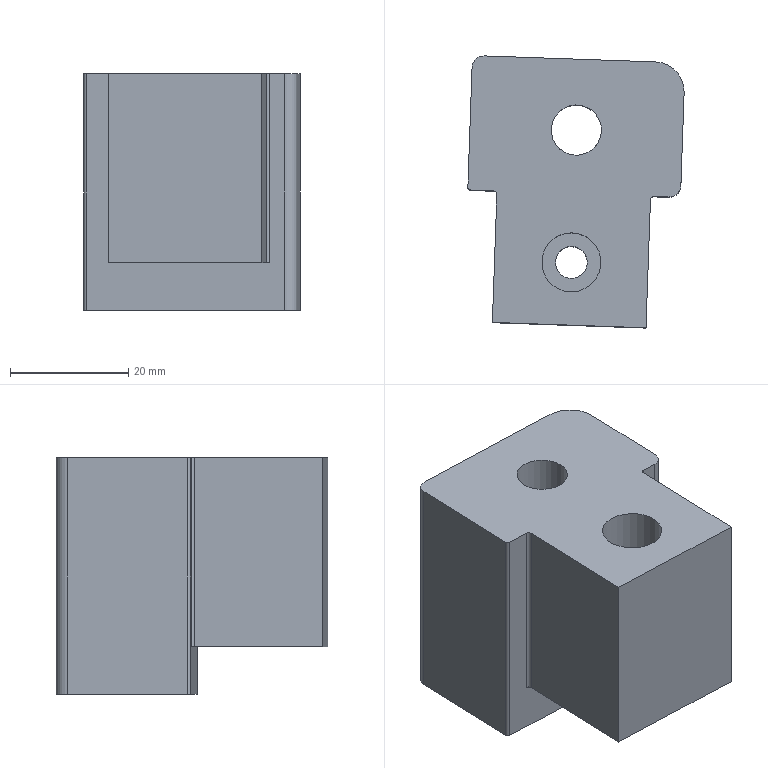Part | NX | features PS-25 2 | 1 solid | 22 faces | box 36.584 x 45.984 x 40 mm | volume 45378 mm3 | plane 12 | cylinder 10 | commonest cylinder face diameters 1 x3 4 x2 10 x2 5.4 x1 8.506 x1 14.5 x1
STEP:
#1=CARTESIAN_POINT('',(3172.903,-916.865,868.716));
#2=VERTEX_POINT('',#1);
#3=CARTESIAN_POINT('',(3198.887,-917.772,868.716));
#4=VERTEX_POINT('',#3);
#5=CARTESIAN_POINT('',(3185.895,-917.319,868.716));
#6=DIRECTION('',(0.9994,-0.0349,0.));
#7=VECTOR('',#6,1000.);
#8=LINE('',#5,#7);
#9=EDGE_CURVE('',#2,#4,#8,.T.);
#10=ORIENTED_EDGE('',*,*,#9,.F.);
#11=CARTESIAN_POINT('',(3173.662,-895.141,868.716));
#12=VERTEX_POINT('',#11);
#13=CARTESIAN_POINT('',(3172.937,-915.898,868.716));
#14=DIRECTION('',(-0.0349,-0.9994,0.));
#15=VECTOR('',#14,1000.);
#16=LINE('',#13,#15);
#17=EDGE_CURVE('',#2,#12,#16,.F.);
#18=ORIENTED_EDGE('',*,*,#17,.T.);
#19=CARTESIAN_POINT('',(3173.179,-894.624,868.716));
#20=VERTEX_POINT('',#19);
#21=CARTESIAN_POINT('',(3173.162,-895.124,868.716));
#22=DIRECTION('',(0.,0.,-1.));
#23=DIRECTION('',(-1.,0.,0.));
#24=AXIS2_PLACEMENT_3D('',#21,#22,#23);
#25=CIRCLE('',#24,0.5);
#26=EDGE_CURVE('',#12,#20,#25,.F.);
#27=ORIENTED_EDGE('',*,*,#26,.T.);
#28=CARTESIAN_POINT('',(3200.163,-895.566,868.716));
#29=VERTEX_POINT('',#28);
#30=CARTESIAN_POINT('',(3186.671,-895.095,868.716));
#31=DIRECTION('',(0.9994,-0.0349,0.));
#32=VECTOR('',#31,1000.);
#33=LINE('',#30,#32);
#34=EDGE_CURVE('',#20,#29,#33,.T.);
#35=ORIENTED_EDGE('',*,*,#34,.T.);
#36=CARTESIAN_POINT('',(3199.646,-896.049,868.716));
#37=VERTEX_POINT('',#36);
#38=CARTESIAN_POINT('',(3200.145,-896.066,868.716));
#39=DIRECTION('',(0.,0.,-1.));
#40=DIRECTION('',(-1.,0.,0.));
#41=AXIS2_PLACEMENT_3D('',#38,#39,#40);
#42=CIRCLE('',#41,0.5);
#43=EDGE_CURVE('',#29,#37,#42,.F.);
#44=ORIENTED_EDGE('',*,*,#43,.T.);
#45=CARTESIAN_POINT('',(3198.921,-916.805,868.716));
#46=DIRECTION('',(0.0349,0.9994,0.));
#47=VECTOR('',#46,1000.);
#48=LINE('',#45,#47);
#49=EDGE_CURVE('',#4,#37,#48,.T.);
#50=ORIENTED_EDGE('',*,*,#49,.F.);
#51=EDGE_LOOP('',(#10,#18,#27,#35,#44,#50));
#52=FACE_BOUND('',#51,.T.);
#53=CARTESIAN_POINT('',(3183.566,-906.707,868.716));
#54=VERTEX_POINT('',#53);
#55=CARTESIAN_POINT('',(3186.266,-906.707,868.716));
#56=DIRECTION('',(0.,0.,-1.));
#57=DIRECTION('',(-1.,0.,0.));
#58=AXIS2_PLACEMENT_3D('',#55,#56,#57);
#59=CIRCLE('',#58,2.7);
#60=EDGE_CURVE('',#54,#54,#59,.F.);
#61=ORIENTED_EDGE('',*,*,#60,.T.);
#62=EDGE_LOOP('',(#61));
#63=FACE_BOUND('',#62,.T.);
#64=CARTESIAN_POINT('',(3186.266,-906.707,868.716));
#65=DIRECTION('',(0.,0.,-1.));
#66=DIRECTION('',(-0.0349,-0.9994,0.));
#67=AXIS2_PLACEMENT_3D('',#64,#65,#66);
#68=PLANE('',#67);
#69=ADVANCED_FACE('',(#52,#63),#68,.T.);
#70=CARTESIAN_POINT('',(3186.266,-911.707,900.716));
#71=VERTEX_POINT('',#70);
#72=CARTESIAN_POINT('',(3186.266,-906.707,900.716));
#73=DIRECTION('',(0.,0.,1.));
#74=DIRECTION('',(0.,-1.,0.));
#75=AXIS2_PLACEMENT_3D('',#72,#73,#74);
#76=CIRCLE('',#75,5.);
#77=EDGE_CURVE('',#71,#71,#76,.T.);
#78=ORIENTED_EDGE('',*,*,#77,.F.);
#79=EDGE_LOOP('',(#78));
#80=FACE_BOUND('',#79,.T.);
#81=CARTESIAN_POINT('',(3200.163,-895.566,900.716));
#82=VERTEX_POINT('',#81);
#83=CARTESIAN_POINT('',(3202.722,-895.656,900.716));
#84=VERTEX_POINT('',#83);
#85=CARTESIAN_POINT('',(3027.832,-889.549,900.716));
#86=DIRECTION('',(-0.9994,0.0349,0.));
#87=VECTOR('',#86,1000.);
#88=LINE('',#85,#87);
#89=EDGE_CURVE('',#82,#84,#88,.F.);
#90=ORIENTED_EDGE('',*,*,#89,.T.);
#91=CARTESIAN_POINT('',(3204.79,-893.727,900.716));
#92=VERTEX_POINT('',#91);
#93=CARTESIAN_POINT('',(3202.792,-893.657,900.716));
#94=DIRECTION('',(0.,0.,1.));
#95=DIRECTION('',(0.,-1.,0.));
#96=AXIS2_PLACEMENT_3D('',#93,#94,#95);
#97=CIRCLE('',#96,2.);
#98=EDGE_CURVE('',#84,#92,#97,.T.);
#99=ORIENTED_EDGE('',*,*,#98,.T.);
#100=CARTESIAN_POINT('',(3205.34,-877.973,900.716));
#101=VERTEX_POINT('',#100);
#102=CARTESIAN_POINT('',(3202.812,-950.375,900.716));
#103=DIRECTION('',(-0.0349,-0.9994,0.));
#104=VECTOR('',#103,1000.);
#105=LINE('',#102,#104);
#106=EDGE_CURVE('',#92,#101,#105,.F.);
#107=ORIENTED_EDGE('',*,*,#106,.T.);
#108=CARTESIAN_POINT('',(3200.518,-872.802,900.716));
#109=VERTEX_POINT('',#108);
#110=CARTESIAN_POINT('',(3200.343,-877.799,900.716));
#111=DIRECTION('',(0.,0.,1.));
#112=DIRECTION('',(0.,-1.,0.));
#113=AXIS2_PLACEMENT_3D('',#110,#111,#112);
#114=CIRCLE('',#113,5.);
#115=EDGE_CURVE('',#109,#101,#114,.F.);
#116=ORIENTED_EDGE('',*,*,#115,.F.);
#117=CARTESIAN_POINT('',(3171.536,-871.79,900.716));
#118=VERTEX_POINT('',#117);
#119=CARTESIAN_POINT('',(3158.544,-871.336,900.716));
#120=DIRECTION('',(-0.9994,0.0349,0.));
#121=VECTOR('',#120,1000.);
#122=LINE('',#119,#121);
#123=EDGE_CURVE('',#109,#118,#122,.T.);
#124=ORIENTED_EDGE('',*,*,#123,.T.);
#125=CARTESIAN_POINT('',(3169.467,-873.719,900.716));
#126=VERTEX_POINT('',#125);
#127=CARTESIAN_POINT('',(3171.466,-873.789,900.716));
#128=DIRECTION('',(0.,0.,1.));
#129=DIRECTION('',(0.,-1.,0.));
#130=AXIS2_PLACEMENT_3D('',#127,#128,#129);
#131=CIRCLE('',#130,2.);
#132=EDGE_CURVE('',#126,#118,#131,.F.);
#133=ORIENTED_EDGE('',*,*,#132,.F.);
#134=CARTESIAN_POINT('',(3168.76,-893.97,900.716));
#135=VERTEX_POINT('',#134);
#136=CARTESIAN_POINT('',(3166.834,-949.119,900.716));
#137=DIRECTION('',(-0.0349,-0.9994,0.));
#138=VECTOR('',#137,1000.);
#139=LINE('',#136,#138);
#140=EDGE_CURVE('',#135,#126,#139,.F.);
#141=ORIENTED_EDGE('',*,*,#140,.F.);
#142=CARTESIAN_POINT('',(3169.242,-894.487,900.716));
#143=VERTEX_POINT('',#142);
#144=CARTESIAN_POINT('',(3169.26,-893.987,900.716));
#145=DIRECTION('',(0.,0.,1.));
#146=DIRECTION('',(0.,-1.,0.));
#147=AXIS2_PLACEMENT_3D('',#144,#145,#146);
#148=CIRCLE('',#147,0.5);
#149=EDGE_CURVE('',#135,#143,#148,.T.);
#150=ORIENTED_EDGE('',*,*,#149,.T.);
#151=CARTESIAN_POINT('',(3173.179,-894.624,900.716));
#152=VERTEX_POINT('',#151);
#153=CARTESIAN_POINT('',(3027.832,-889.549,900.716));
#154=DIRECTION('',(-0.9994,0.0349,0.));
#155=VECTOR('',#154,1000.);
#156=LINE('',#153,#155);
#157=EDGE_CURVE('',#143,#152,#156,.F.);
#158=ORIENTED_EDGE('',*,*,#157,.T.);
#159=CARTESIAN_POINT('',(3173.662,-895.141,900.716));
#160=VERTEX_POINT('',#159);
#161=CARTESIAN_POINT('',(3173.162,-895.124,900.716));
#162=DIRECTION('',(0.,0.,1.));
#163=DIRECTION('',(0.,-1.,0.));
#164=AXIS2_PLACEMENT_3D('',#161,#162,#163);
#165=CIRCLE('',#164,0.5);
#166=EDGE_CURVE('',#152,#160,#165,.F.);
#167=ORIENTED_EDGE('',*,*,#166,.T.);
#168=CARTESIAN_POINT('',(3172.903,-916.865,900.716));
#169=VERTEX_POINT('',#168);
#170=CARTESIAN_POINT('',(3172.937,-915.898,900.716));
#171=DIRECTION('',(0.0349,0.9994,0.));
#172=VECTOR('',#171,1000.);
#173=LINE('',#170,#172);
#174=EDGE_CURVE('',#169,#160,#173,.T.);
#175=ORIENTED_EDGE('',*,*,#174,.F.);
#176=CARTESIAN_POINT('',(3198.887,-917.772,900.716));
#177=VERTEX_POINT('',#176);
#178=CARTESIAN_POINT('',(3027.056,-911.773,900.716));
#179=DIRECTION('',(-0.9994,0.0349,0.));
#180=VECTOR('',#179,1000.);
#181=LINE('',#178,#180);
#182=EDGE_CURVE('',#169,#177,#181,.F.);
#183=ORIENTED_EDGE('',*,*,#182,.T.);
#184=CARTESIAN_POINT('',(3199.646,-896.049,900.716));
#185=VERTEX_POINT('',#184);
#186=CARTESIAN_POINT('',(3198.921,-916.805,900.716));
#187=DIRECTION('',(-0.0349,-0.9994,0.));
#188=VECTOR('',#187,1000.);
#189=LINE('',#186,#188);
#190=EDGE_CURVE('',#177,#185,#189,.F.);
#191=ORIENTED_EDGE('',*,*,#190,.T.);
#192=CARTESIAN_POINT('',(3200.145,-896.066,900.716));
#193=DIRECTION('',(0.,0.,1.));
#194=DIRECTION('',(0.,-1.,0.));
#195=AXIS2_PLACEMENT_3D('',#192,#193,#194);
#196=CIRCLE('',#195,0.5);
#197=EDGE_CURVE('',#185,#82,#196,.F.);
#198=ORIENTED_EDGE('',*,*,#197,.T.);
#199=EDGE_LOOP('',(#90,#99,#107,#116,#124,#133,#141,#150,#158,#167,#175,#183,#191,#198));
#200=FACE_BOUND('',#199,.T.);
#201=CARTESIAN_POINT('',(3187.107,-888.594,900.716));
#202=VERTEX_POINT('',#201);
#203=CARTESIAN_POINT('',(3187.107,-884.341,900.716));
#204=DIRECTION('',(0.,0.,1.));
#205=DIRECTION('',(0.,-1.,0.));
#206=AXIS2_PLACEMENT_3D('',#203,#204,#205);
#207=CIRCLE('',#206,4.253);
#208=EDGE_CURVE('',#202,#202,#207,.T.);
#209=ORIENTED_EDGE('',*,*,#208,.F.);
#210=EDGE_LOOP('',(#209));
#211=FACE_BOUND('',#210,.T.);
#212=CARTESIAN_POINT('',(3025.924,-944.199,900.716));
#213=DIRECTION('',(0.,0.,1.));
#214=DIRECTION('',(0.9976,-0.06975,0.));
#215=AXIS2_PLACEMENT_3D('',#212,#213,#214);
#216=PLANE('',#215);
#217=ADVANCED_FACE('',(#80,#200,#211),#216,.T.);
#218=ORIENTED_EDGE('',*,*,#49,.T.);
#219=CARTESIAN_POINT('',(3199.646,-896.049,830.716));
#220=DIRECTION('',(0.,0.,1.));
#221=VECTOR('',#220,1000.);
#222=LINE('',#219,#221);
#223=EDGE_CURVE('',#37,#185,#222,.T.);
#224=ORIENTED_EDGE('',*,*,#223,.T.);
#225=ORIENTED_EDGE('',*,*,#190,.F.);
#226=CARTESIAN_POINT('',(3198.887,-917.772,880.716));
#227=DIRECTION('',(0.,0.,-1.));
#228=VECTOR('',#227,1000.);
#229=LINE('',#226,#228);
#230=EDGE_CURVE('',#177,#4,#229,.T.);
#231=ORIENTED_EDGE('',*,*,#230,.T.);
#232=EDGE_LOOP('',(#218,#224,#225,#231));
#233=FACE_BOUND('',#232,.T.);
#234=CARTESIAN_POINT('',(3198.921,-916.805,830.716));
#235=DIRECTION('',(0.9994,-0.0349,0.));
#236=DIRECTION('',(0.0349,0.9994,0.));
#237=AXIS2_PLACEMENT_3D('',#234,#235,#236);
#238=PLANE('',#237);
#239=ADVANCED_FACE('',(#233),#238,.T.);
#240=ORIENTED_EDGE('',*,*,#17,.F.);
#241=CARTESIAN_POINT('',(3172.903,-916.865,830.716));
#242=DIRECTION('',(0.,0.,-1.));
#243=VECTOR('',#242,1000.);
#244=LINE('',#241,#243);
#245=EDGE_CURVE('',#169,#2,#244,.T.);
#246=ORIENTED_EDGE('',*,*,#245,.F.);
#247=ORIENTED_EDGE('',*,*,#174,.T.);
#248=CARTESIAN_POINT('',(3173.662,-895.141,863.216));
#249=DIRECTION('',(0.,0.,1.));
#250=VECTOR('',#249,1000.);
#251=LINE('',#248,#250);
#252=EDGE_CURVE('',#160,#12,#251,.F.);
#253=ORIENTED_EDGE('',*,*,#252,.T.);
#254=EDGE_LOOP('',(#240,#246,#247,#253));
#255=FACE_BOUND('',#254,.T.);
#256=CARTESIAN_POINT('',(3172.937,-915.898,830.716));
#257=DIRECTION('',(-0.9994,0.0349,0.));
#258=DIRECTION('',(-0.0349,-0.9994,0.));
#259=AXIS2_PLACEMENT_3D('',#256,#257,#258);
#260=PLANE('',#259);
#261=ADVANCED_FACE('',(#255),#260,.T.);
#262=CARTESIAN_POINT('',(3186.266,-901.707,890.716));
#263=VERTEX_POINT('',#262);
#264=CARTESIAN_POINT('',(3186.266,-906.707,890.716));
#265=DIRECTION('',(0.,0.,-1.));
#266=DIRECTION('',(0.,1.,0.));
#267=AXIS2_PLACEMENT_3D('',#264,#265,#266);
#268=CIRCLE('',#267,5.);
#269=EDGE_CURVE('',#263,#263,#268,.F.);
#270=ORIENTED_EDGE('',*,*,#269,.F.);
#271=EDGE_LOOP('',(#270));
#272=FACE_BOUND('',#271,.T.);
#273=ORIENTED_EDGE('',*,*,#77,.T.);
#274=EDGE_LOOP('',(#273));
#275=FACE_BOUND('',#274,.T.);
#276=CARTESIAN_POINT('',(3186.266,-906.707,935.716));
#277=DIRECTION('',(0.,0.,-1.));
#278=DIRECTION('',(0.9976,-0.06975,0.));
#279=AXIS2_PLACEMENT_3D('',#276,#277,#278);
#280=CYLINDRICAL_SURFACE('',#279,5.);
#281=ADVANCED_FACE('',(#272,#275),#280,.F.);
#282=ORIENTED_EDGE('',*,*,#60,.F.);
#283=EDGE_LOOP('',(#282));
#284=FACE_BOUND('',#283,.T.);
#285=CARTESIAN_POINT('',(3186.266,-904.007,890.716));
#286=VERTEX_POINT('',#285);
#287=CARTESIAN_POINT('',(3186.266,-906.707,890.716));
#288=DIRECTION('',(0.,0.,-1.));
#289=DIRECTION('',(0.,1.,0.));
#290=AXIS2_PLACEMENT_3D('',#287,#288,#289);
#291=CIRCLE('',#290,2.7);
#292=EDGE_CURVE('',#286,#286,#291,.T.);
#293=ORIENTED_EDGE('',*,*,#292,.F.);
#294=EDGE_LOOP('',(#293));
#295=FACE_BOUND('',#294,.T.);
#296=CARTESIAN_POINT('',(3186.266,-906.707,872.716));
#297=DIRECTION('',(0.,0.,-1.));
#298=DIRECTION('',(0.9976,-0.06975,0.));
#299=AXIS2_PLACEMENT_3D('',#296,#297,#298);
#300=CYLINDRICAL_SURFACE('',#299,2.7);
#301=ADVANCED_FACE('',(#284,#295),#300,.F.);
#302=ORIENTED_EDGE('',*,*,#292,.T.);
#303=EDGE_LOOP('',(#302));
#304=FACE_BOUND('',#303,.T.);
#305=ORIENTED_EDGE('',*,*,#269,.T.);
#306=EDGE_LOOP('',(#305));
#307=FACE_BOUND('',#306,.T.);
#308=CARTESIAN_POINT('',(3186.266,-906.707,890.716));
#309=DIRECTION('',(0.,0.,-1.));
#310=DIRECTION('',(-0.9976,0.06975,0.));
#311=AXIS2_PLACEMENT_3D('',#308,#309,#310);
#312=PLANE('',#311);
#313=ADVANCED_FACE('',(#304,#307),#312,.F.);
#314=ORIENTED_EDGE('',*,*,#197,.F.);
#315=ORIENTED_EDGE('',*,*,#223,.F.);
#316=ORIENTED_EDGE('',*,*,#43,.F.);
#317=CARTESIAN_POINT('',(3200.163,-895.566,863.216));
#318=DIRECTION('',(0.,0.,1.));
#319=VECTOR('',#318,1000.);
#320=LINE('',#317,#319);
#321=EDGE_CURVE('',#82,#29,#320,.F.);
#322=ORIENTED_EDGE('',*,*,#321,.F.);
#323=EDGE_LOOP('',(#314,#315,#316,#322));
#324=FACE_BOUND('',#323,.T.);
#325=CARTESIAN_POINT('',(3200.145,-896.066,830.716));
#326=DIRECTION('',(0.,0.,1.));
#327=DIRECTION('',(0.,-1.,0.));
#328=AXIS2_PLACEMENT_3D('',#325,#326,#327);
#329=CYLINDRICAL_SURFACE('',#328,0.5);
#330=ADVANCED_FACE('',(#324),#329,.F.);
#331=ORIENTED_EDGE('',*,*,#166,.F.);
#332=CARTESIAN_POINT('',(3173.179,-894.624,863.216));
#333=DIRECTION('',(0.,0.,-1.));
#334=VECTOR('',#333,1000.);
#335=LINE('',#332,#334);
#336=EDGE_CURVE('',#20,#152,#335,.F.);
#337=ORIENTED_EDGE('',*,*,#336,.F.);
#338=ORIENTED_EDGE('',*,*,#26,.F.);
#339=ORIENTED_EDGE('',*,*,#252,.F.);
#340=EDGE_LOOP('',(#331,#337,#338,#339));
#341=FACE_BOUND('',#340,.T.);
#342=CARTESIAN_POINT('',(3173.162,-895.124,863.216));
#343=DIRECTION('',(0.,0.,1.));
#344=DIRECTION('',(0.,-1.,0.));
#345=AXIS2_PLACEMENT_3D('',#342,#343,#344);
#346=CYLINDRICAL_SURFACE('',#345,0.5);
#347=ADVANCED_FACE('',(#341),#346,.F.);
#348=CARTESIAN_POINT('',(3202.722,-895.656,860.716));
#349=VERTEX_POINT('',#348);
#350=CARTESIAN_POINT('',(3169.242,-894.487,860.716));
#351=VERTEX_POINT('',#350);
#352=CARTESIAN_POINT('',(2864.273,-883.838,860.716));
#353=DIRECTION('',(0.9994,-0.0349,0.));
#354=VECTOR('',#353,1000.);
#355=LINE('',#352,#354);
#356=EDGE_CURVE('',#349,#351,#355,.F.);
#357=ORIENTED_EDGE('',*,*,#356,.F.);
#358=CARTESIAN_POINT('',(3202.722,-895.656,900.716));
#359=DIRECTION('',(0.,0.,1.));
#360=VECTOR('',#359,1000.);
#361=LINE('',#358,#360);
#362=EDGE_CURVE('',#349,#84,#361,.T.);
#363=ORIENTED_EDGE('',*,*,#362,.T.);
#364=ORIENTED_EDGE('',*,*,#89,.F.);
#365=ORIENTED_EDGE('',*,*,#321,.T.);
#366=ORIENTED_EDGE('',*,*,#34,.F.);
#367=ORIENTED_EDGE('',*,*,#336,.T.);
#368=ORIENTED_EDGE('',*,*,#157,.F.);
#369=CARTESIAN_POINT('',(3169.242,-894.487,863.216));
#370=DIRECTION('',(0.,0.,1.));
#371=VECTOR('',#370,1000.);
#372=LINE('',#369,#371);
#373=EDGE_CURVE('',#143,#351,#372,.F.);
#374=ORIENTED_EDGE('',*,*,#373,.T.);
#375=EDGE_LOOP('',(#357,#363,#364,#365,#366,#367,#368,#374));
#376=FACE_BOUND('',#375,.T.);
#377=CARTESIAN_POINT('',(3183.542,-894.986,863.216));
#378=DIRECTION('',(0.0349,0.9994,0.));
#379=DIRECTION('',(-0.9994,0.0349,0.));
#380=AXIS2_PLACEMENT_3D('',#377,#378,#379);
#381=PLANE('',#380);
#382=ADVANCED_FACE('',(#376),#381,.F.);
#383=CARTESIAN_POINT('',(3191.35,-884.638,879.716));
#384=VERTEX_POINT('',#383);
#385=CARTESIAN_POINT('',(3187.107,-884.341,879.716));
#386=DIRECTION('',(0.,0.,-1.));
#387=DIRECTION('',(0.9976,-0.06975,0.));
#388=AXIS2_PLACEMENT_3D('',#385,#386,#387);
#389=CIRCLE('',#388,4.253);
#390=EDGE_CURVE('',#384,#384,#389,.T.);
#391=ORIENTED_EDGE('',*,*,#390,.F.);
#392=EDGE_LOOP('',(#391));
#393=FACE_BOUND('',#392,.T.);
#394=CARTESIAN_POINT('',(3194.339,-884.847,879.716));
#395=VERTEX_POINT('',#394);
#396=CARTESIAN_POINT('',(3187.107,-884.341,879.716));
#397=DIRECTION('',(0.,0.,1.));
#398=DIRECTION('',(0.9976,-0.06975,0.));
#399=AXIS2_PLACEMENT_3D('',#396,#397,#398);
#400=CIRCLE('',#399,7.25);
#401=EDGE_CURVE('',#395,#395,#400,.F.);
#402=ORIENTED_EDGE('',*,*,#401,.T.);
#403=EDGE_LOOP('',(#402));
#404=FACE_BOUND('',#403,.T.);
#405=CARTESIAN_POINT('',(3187.107,-884.341,879.716));
#406=DIRECTION('',(0.,0.,1.));
#407=DIRECTION('',(0.9976,-0.06975,0.));
#408=AXIS2_PLACEMENT_3D('',#405,#406,#407);
#409=PLANE('',#408);
#410=ADVANCED_FACE('',(#393,#404),#409,.F.);
#411=ORIENTED_EDGE('',*,*,#390,.T.);
#412=EDGE_LOOP('',(#411));
#413=FACE_BOUND('',#412,.T.);
#414=ORIENTED_EDGE('',*,*,#208,.T.);
#415=EDGE_LOOP('',(#414));
#416=FACE_BOUND('',#415,.T.);
#417=CARTESIAN_POINT('',(3187.107,-884.341,868.716));
#418=DIRECTION('',(0.,0.,1.));
#419=DIRECTION('',(0.9976,-0.06975,0.));
#420=AXIS2_PLACEMENT_3D('',#417,#418,#419);
#421=CYLINDRICAL_SURFACE('',#420,4.253);
#422=ADVANCED_FACE('',(#413,#416),#421,.F.);
#423=CARTESIAN_POINT('',(3168.76,-893.97,860.716));
#424=VERTEX_POINT('',#423);
#425=CARTESIAN_POINT('',(3169.26,-893.987,860.716));
#426=DIRECTION('',(0.,0.,-1.));
#427=DIRECTION('',(1.,0.,0.));
#428=AXIS2_PLACEMENT_3D('',#425,#426,#427);
#429=CIRCLE('',#428,0.5);
#430=EDGE_CURVE('',#351,#424,#429,.T.);
#431=ORIENTED_EDGE('',*,*,#430,.F.);
#432=ORIENTED_EDGE('',*,*,#373,.F.);
#433=ORIENTED_EDGE('',*,*,#149,.F.);
#434=CARTESIAN_POINT('',(3168.76,-893.97,890.716));
#435=DIRECTION('',(0.,0.,1.));
#436=VECTOR('',#435,1000.);
#437=LINE('',#434,#436);
#438=EDGE_CURVE('',#424,#135,#437,.T.);
#439=ORIENTED_EDGE('',*,*,#438,.F.);
#440=EDGE_LOOP('',(#431,#432,#433,#439));
#441=FACE_BOUND('',#440,.T.);
#442=CARTESIAN_POINT('',(3169.26,-893.987,890.716));
#443=DIRECTION('',(0.,0.,1.));
#444=DIRECTION('',(1.,0.,0.));
#445=AXIS2_PLACEMENT_3D('',#442,#443,#444);
#446=CYLINDRICAL_SURFACE('',#445,0.5);
#447=ADVANCED_FACE('',(#441),#446,.T.);
#448=CARTESIAN_POINT('',(3169.467,-873.719,860.716));
#449=VERTEX_POINT('',#448);
#450=CARTESIAN_POINT('',(3174.564,-727.754,860.716));
#451=DIRECTION('',(-0.0349,-0.9994,0.));
#452=VECTOR('',#451,1000.);
#453=LINE('',#450,#452);
#454=EDGE_CURVE('',#424,#449,#453,.F.);
#455=ORIENTED_EDGE('',*,*,#454,.F.);
#456=ORIENTED_EDGE('',*,*,#438,.T.);
#457=ORIENTED_EDGE('',*,*,#140,.T.);
#458=CARTESIAN_POINT('',(3169.467,-873.719,890.716));
#459=DIRECTION('',(0.,0.,1.));
#460=VECTOR('',#459,1000.);
#461=LINE('',#458,#460);
#462=EDGE_CURVE('',#449,#126,#461,.T.);
#463=ORIENTED_EDGE('',*,*,#462,.F.);
#464=EDGE_LOOP('',(#455,#456,#457,#463));
#465=FACE_BOUND('',#464,.T.);
#466=CARTESIAN_POINT('',(3168.523,-900.744,890.716));
#467=DIRECTION('',(0.9994,-0.0349,0.));
#468=DIRECTION('',(-0.0349,-0.9994,0.));
#469=AXIS2_PLACEMENT_3D('',#466,#467,#468);
#470=PLANE('',#469);
#471=ADVANCED_FACE('',(#465),#470,.F.);
#472=ORIENTED_EDGE('',*,*,#132,.T.);
#473=CARTESIAN_POINT('',(3171.536,-871.79,860.716));
#474=VERTEX_POINT('',#473);
#475=CARTESIAN_POINT('',(3171.536,-871.79,860.716));
#476=DIRECTION('',(0.,0.,-1.));
#477=VECTOR('',#476,1000.);
#478=LINE('',#475,#477);
#479=EDGE_CURVE('',#118,#474,#478,.T.);
#480=ORIENTED_EDGE('',*,*,#479,.T.);
#481=CARTESIAN_POINT('',(3171.466,-873.789,860.716));
#482=DIRECTION('',(0.,0.,-1.));
#483=DIRECTION('',(1.,0.,0.));
#484=AXIS2_PLACEMENT_3D('',#481,#482,#483);
#485=CIRCLE('',#484,2.);
#486=EDGE_CURVE('',#474,#449,#485,.F.);
#487=ORIENTED_EDGE('',*,*,#486,.T.);
#488=ORIENTED_EDGE('',*,*,#462,.T.);
#489=EDGE_LOOP('',(#472,#480,#487,#488));
#490=FACE_BOUND('',#489,.T.);
#491=CARTESIAN_POINT('',(3171.466,-873.789,935.716));
#492=DIRECTION('',(0.,0.,-1.));
#493=DIRECTION('',(-0.9976,0.06975,0.));
#494=AXIS2_PLACEMENT_3D('',#491,#492,#493);
#495=CYLINDRICAL_SURFACE('',#494,2.);
#496=ADVANCED_FACE('',(#490),#495,.T.);
#497=CARTESIAN_POINT('',(3200.518,-872.802,860.716));
#498=VERTEX_POINT('',#497);
#499=CARTESIAN_POINT('',(3158.544,-871.336,860.716));
#500=DIRECTION('',(0.9994,-0.0349,0.));
#501=VECTOR('',#500,1000.);
#502=LINE('',#499,#501);
#503=EDGE_CURVE('',#474,#498,#502,.T.);
#504=ORIENTED_EDGE('',*,*,#503,.F.);
#505=ORIENTED_EDGE('',*,*,#479,.F.);
#506=ORIENTED_EDGE('',*,*,#123,.F.);
#507=CARTESIAN_POINT('',(3200.518,-872.802,935.716));
#508=DIRECTION('',(0.,0.,-1.));
#509=VECTOR('',#508,1000.);
#510=LINE('',#507,#509);
#511=EDGE_CURVE('',#498,#109,#510,.F.);
#512=ORIENTED_EDGE('',*,*,#511,.F.);
#513=EDGE_LOOP('',(#504,#505,#506,#512));
#514=FACE_BOUND('',#513,.T.);
#515=CARTESIAN_POINT('',(3158.544,-871.336,935.716));
#516=DIRECTION('',(-0.0349,-0.9994,0.));
#517=DIRECTION('',(-0.9994,0.0349,0.));
#518=AXIS2_PLACEMENT_3D('',#515,#516,#517);
#519=PLANE('',#518);
#520=ADVANCED_FACE('',(#514),#519,.F.);
#521=ORIENTED_EDGE('',*,*,#115,.T.);
#522=CARTESIAN_POINT('',(3205.34,-877.973,860.716));
#523=VERTEX_POINT('',#522);
#524=CARTESIAN_POINT('',(3205.34,-877.973,862.716));
#525=DIRECTION('',(0.,0.,1.));
#526=VECTOR('',#525,1000.);
#527=LINE('',#524,#526);
#528=EDGE_CURVE('',#101,#523,#527,.F.);
#529=ORIENTED_EDGE('',*,*,#528,.T.);
#530=CARTESIAN_POINT('',(3200.343,-877.799,860.716));
#531=DIRECTION('',(0.,0.,-1.));
#532=DIRECTION('',(1.,0.,0.));
#533=AXIS2_PLACEMENT_3D('',#530,#531,#532);
#534=CIRCLE('',#533,5.);
#535=EDGE_CURVE('',#523,#498,#534,.F.);
#536=ORIENTED_EDGE('',*,*,#535,.T.);
#537=ORIENTED_EDGE('',*,*,#511,.T.);
#538=EDGE_LOOP('',(#521,#529,#536,#537));
#539=FACE_BOUND('',#538,.T.);
#540=CARTESIAN_POINT('',(3200.343,-877.799,862.716));
#541=DIRECTION('',(0.,0.,1.));
#542=DIRECTION('',(0.9976,-0.06975,0.));
#543=AXIS2_PLACEMENT_3D('',#540,#541,#542);
#544=CYLINDRICAL_SURFACE('',#543,5.);
#545=ADVANCED_FACE('',(#539),#544,.T.);
#546=ORIENTED_EDGE('',*,*,#106,.F.);
#547=CARTESIAN_POINT('',(3204.79,-893.727,860.716));
#548=VERTEX_POINT('',#547);
#549=CARTESIAN_POINT('',(3204.79,-893.727,860.716));
#550=DIRECTION('',(0.,0.,1.));
#551=VECTOR('',#550,1000.);
#552=LINE('',#549,#551);
#553=EDGE_CURVE('',#92,#548,#552,.F.);
#554=ORIENTED_EDGE('',*,*,#553,.T.);
#555=CARTESIAN_POINT('',(3210.542,-729.01,860.716));
#556=DIRECTION('',(-0.0349,-0.9994,0.));
#557=VECTOR('',#556,1000.);
#558=LINE('',#555,#557);
#559=EDGE_CURVE('',#548,#523,#558,.F.);
#560=ORIENTED_EDGE('',*,*,#559,.T.);
#561=ORIENTED_EDGE('',*,*,#528,.F.);
#562=EDGE_LOOP('',(#546,#554,#560,#561));
#563=FACE_BOUND('',#562,.T.);
#564=CARTESIAN_POINT('',(3204.536,-901.001,862.716));
#565=DIRECTION('',(0.9994,-0.0349,0.));
#566=DIRECTION('',(-0.0349,-0.9994,0.));
#567=AXIS2_PLACEMENT_3D('',#564,#565,#566);
#568=PLANE('',#567);
#569=ADVANCED_FACE('',(#563),#568,.T.);
#570=ORIENTED_EDGE('',*,*,#401,.F.);
#571=EDGE_LOOP('',(#570));
#572=FACE_BOUND('',#571,.T.);
#573=CARTESIAN_POINT('',(3194.357,-884.341,860.716));
#574=VERTEX_POINT('',#573);
#575=CARTESIAN_POINT('',(3187.107,-884.341,860.716));
#576=DIRECTION('',(0.,0.,-1.));
#577=DIRECTION('',(1.,0.,0.));
#578=AXIS2_PLACEMENT_3D('',#575,#576,#577);
#579=CIRCLE('',#578,7.25);
#580=EDGE_CURVE('',#574,#574,#579,.T.);
#581=ORIENTED_EDGE('',*,*,#580,.T.);
#582=EDGE_LOOP('',(#581));
#583=FACE_BOUND('',#582,.T.);
#584=CARTESIAN_POINT('',(3187.107,-884.341,868.716));
#585=DIRECTION('',(0.,0.,1.));
#586=DIRECTION('',(0.9976,-0.06975,0.));
#587=AXIS2_PLACEMENT_3D('',#584,#585,#586);
#588=CYLINDRICAL_SURFACE('',#587,7.25);
#589=ADVANCED_FACE('',(#572,#583),#588,.F.);
#590=ORIENTED_EDGE('',*,*,#580,.F.);
#591=EDGE_LOOP('',(#590));
#592=FACE_BOUND('',#591,.T.);
#593=ORIENTED_EDGE('',*,*,#559,.F.);
#594=CARTESIAN_POINT('',(3202.792,-893.657,860.716));
#595=DIRECTION('',(0.,0.,1.));
#596=DIRECTION('',(1.,0.,0.));
#597=AXIS2_PLACEMENT_3D('',#594,#595,#596);
#598=CIRCLE('',#597,2.);
#599=EDGE_CURVE('',#548,#349,#598,.F.);
#600=ORIENTED_EDGE('',*,*,#599,.T.);
#601=ORIENTED_EDGE('',*,*,#356,.T.);
#602=ORIENTED_EDGE('',*,*,#430,.T.);
#603=ORIENTED_EDGE('',*,*,#454,.T.);
#604=ORIENTED_EDGE('',*,*,#486,.F.);
#605=ORIENTED_EDGE('',*,*,#503,.T.);
#606=ORIENTED_EDGE('',*,*,#535,.F.);
#607=EDGE_LOOP('',(#593,#600,#601,#602,#603,#604,#605,#606));
#608=FACE_BOUND('',#607,.T.);
#609=CARTESIAN_POINT('',(2870.094,-717.123,860.716));
#610=DIRECTION('',(0.,0.,1.));
#611=DIRECTION('',(0.,-1.,0.));
#612=AXIS2_PLACEMENT_3D('',#609,#610,#611);
#613=PLANE('',#612);
#614=ADVANCED_FACE('',(#592,#608),#613,.F.);
#615=ORIENTED_EDGE('',*,*,#9,.T.);
#616=ORIENTED_EDGE('',*,*,#230,.F.);
#617=ORIENTED_EDGE('',*,*,#182,.F.);
#618=ORIENTED_EDGE('',*,*,#245,.T.);
#619=EDGE_LOOP('',(#615,#616,#617,#618));
#620=FACE_BOUND('',#619,.T.);
#621=CARTESIAN_POINT('',(3183.957,-917.251,880.716));
#622=DIRECTION('',(0.0349,0.9994,0.));
#623=DIRECTION('',(-0.9994,0.0349,0.));
#624=AXIS2_PLACEMENT_3D('',#621,#622,#623);
#625=PLANE('',#624);
#626=ADVANCED_FACE('',(#620),#625,.F.);
#627=ORIENTED_EDGE('',*,*,#599,.F.);
#628=ORIENTED_EDGE('',*,*,#553,.F.);
#629=ORIENTED_EDGE('',*,*,#98,.F.);
#630=ORIENTED_EDGE('',*,*,#362,.F.);
#631=EDGE_LOOP('',(#627,#628,#629,#630));
#632=FACE_BOUND('',#631,.T.);
#633=CARTESIAN_POINT('',(3202.792,-893.657,863.216));
#634=DIRECTION('',(0.,0.,-1.));
#635=DIRECTION('',(-1.,0.,0.));
#636=AXIS2_PLACEMENT_3D('',#633,#634,#635);
#637=CYLINDRICAL_SURFACE('',#636,2.);
#638=ADVANCED_FACE('',(#632),#637,.T.);
#639=CLOSED_SHELL('',(#69,#217,#239,#261,#281,#301,#313,#330,#347,#382,#410,#422,#447,#471,#496,#520,#545,#569,#589,#614,#626,#638));
#640=MANIFOLD_SOLID_BREP('',#639);
#641=(LENGTH_UNIT()NAMED_UNIT(*)SI_UNIT(.MILLI.,.METRE.));
#642=UNCERTAINTY_MEASURE_WITH_UNIT(LENGTH_MEASURE(0.00001),#641,'','');
#643=(NAMED_UNIT(*)PLANE_ANGLE_UNIT()SI_UNIT($,.RADIAN.));
#644=(NAMED_UNIT(*)SI_UNIT($,.STERADIAN.)SOLID_ANGLE_UNIT());
#645=(GEOMETRIC_REPRESENTATION_CONTEXT(3)GLOBAL_UNCERTAINTY_ASSIGNED_CONTEXT((#642))GLOBAL_UNIT_ASSIGNED_CONTEXT((#641,#643,#644))REPRESENTATION_CONTEXT('',''));
#646=ADVANCED_BREP_SHAPE_REPRESENTATION('',(#640),#645);